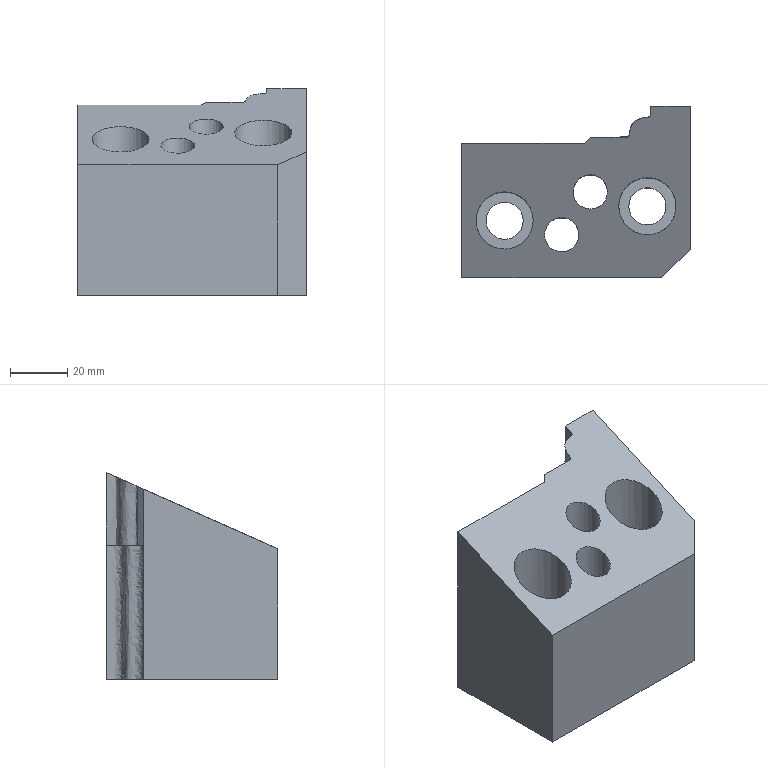Part | NX | features solid 2 | 1 solid | 20 faces | box 80 x 60 x 72.376 mm | volume 180739 mm3 | plane 11 | cylinder 6 | spline 3 | commonest cylinder face diameters 12 x2 13 x2 20 x2
STEP:
#1=CARTESIAN_POINT('',(-526.5,770.,-210.));
#2=VERTEX_POINT('',#1);
#3=CARTESIAN_POINT('',(-533.,770.,-210.));
#4=DIRECTION('',(0.,0.,1.));
#5=DIRECTION('',(1.,0.,0.));
#6=AXIS2_PLACEMENT_3D('',#3,#4,#5);
#7=CIRCLE('',#6,6.5);
#8=EDGE_CURVE('',#2,#2,#7,.F.);
#9=ORIENTED_EDGE('',*,*,#8,.F.);
#10=EDGE_LOOP('',(#9));
#11=FACE_BOUND('',#10,.T.);
#12=CARTESIAN_POINT('',(-476.5,775.,-210.));
#13=VERTEX_POINT('',#12);
#14=CARTESIAN_POINT('',(-483.,775.,-210.));
#15=DIRECTION('',(0.,0.,1.));
#16=DIRECTION('',(1.,0.,0.));
#17=AXIS2_PLACEMENT_3D('',#14,#15,#16);
#18=CIRCLE('',#17,6.5);
#19=EDGE_CURVE('',#13,#13,#18,.F.);
#20=ORIENTED_EDGE('',*,*,#19,.F.);
#21=EDGE_LOOP('',(#20));
#22=FACE_BOUND('',#21,.T.);
#23=CARTESIAN_POINT('',(-497.,780.,-210.));
#24=VERTEX_POINT('',#23);
#25=CARTESIAN_POINT('',(-503.,780.,-210.));
#26=DIRECTION('',(0.,0.,1.));
#27=DIRECTION('',(1.,0.,0.));
#28=AXIS2_PLACEMENT_3D('',#25,#26,#27);
#29=CIRCLE('',#28,6.);
#30=EDGE_CURVE('',#24,#24,#29,.T.);
#31=ORIENTED_EDGE('',*,*,#30,.T.);
#32=EDGE_LOOP('',(#31));
#33=FACE_BOUND('',#32,.T.);
#34=CARTESIAN_POINT('',(-507.,765.,-210.));
#35=VERTEX_POINT('',#34);
#36=CARTESIAN_POINT('',(-513.,765.,-210.));
#37=DIRECTION('',(0.,0.,1.));
#38=DIRECTION('',(1.,0.,0.));
#39=AXIS2_PLACEMENT_3D('',#36,#37,#38);
#40=CIRCLE('',#39,6.);
#41=EDGE_CURVE('',#35,#35,#40,.T.);
#42=ORIENTED_EDGE('',*,*,#41,.T.);
#43=EDGE_LOOP('',(#42));
#44=FACE_BOUND('',#43,.T.);
#45=CARTESIAN_POINT('',(-479.634,810.,-210.));
#46=VERTEX_POINT('',#45);
#47=CARTESIAN_POINT('',(-505.156,797.,-210.));
#48=VERTEX_POINT('',#47);
#49=CARTESIAN_POINT('',(-505.156,797.,-210.));
#50=CARTESIAN_POINT('',(-501.176,797.,-210.));
#51=CARTESIAN_POINT('',(-497.196,797.,-210.));
#52=CARTESIAN_POINT('',(-493.216,797.,-210.));
#53=CARTESIAN_POINT('',(-492.832,797.,-210.));
#54=CARTESIAN_POINT('',(-492.076,797.002,-210.));
#55=CARTESIAN_POINT('',(-491.171,796.978,-210.));
#56=CARTESIAN_POINT('',(-490.387,796.991,-210.));
#57=CARTESIAN_POINT('',(-490.095,797.005,-210.));
#58=CARTESIAN_POINT('',(-489.739,797.026,-210.));
#59=CARTESIAN_POINT('',(-489.186,797.163,-210.));
#60=CARTESIAN_POINT('',(-488.37,797.523,-210.));
#61=CARTESIAN_POINT('',(-487.599,798.274,-210.));
#62=CARTESIAN_POINT('',(-487.195,799.181,-210.));
#63=CARTESIAN_POINT('',(-487.08,799.817,-210.));
#64=CARTESIAN_POINT('',(-487.037,800.426,-210.));
#65=CARTESIAN_POINT('',(-486.999,801.092,-210.));
#66=CARTESIAN_POINT('',(-486.838,801.902,-210.));
#67=CARTESIAN_POINT('',(-486.363,802.737,-210.));
#68=CARTESIAN_POINT('',(-485.47,803.365,-210.));
#69=CARTESIAN_POINT('',(-484.448,803.704,-210.));
#70=CARTESIAN_POINT('',(-483.835,803.806,-210.));
#71=CARTESIAN_POINT('',(-483.198,803.851,-210.));
#72=CARTESIAN_POINT('',(-482.731,803.897,-210.));
#73=CARTESIAN_POINT('',(-482.41,803.93,-210.));
#74=CARTESIAN_POINT('',(-481.63,804.089,-210.));
#75=CARTESIAN_POINT('',(-480.777,804.582,-210.));
#76=CARTESIAN_POINT('',(-480.157,805.239,-210.));
#77=CARTESIAN_POINT('',(-479.718,806.198,-210.));
#78=CARTESIAN_POINT('',(-479.64,806.858,-210.));
#79=CARTESIAN_POINT('',(-479.609,807.399,-210.));
#80=CARTESIAN_POINT('',(-479.625,808.001,-210.));
#81=CARTESIAN_POINT('',(-479.634,808.486,-210.));
#82=CARTESIAN_POINT('',(-479.634,808.867,-210.));
#83=CARTESIAN_POINT('',(-479.634,809.059,-210.));
#84=CARTESIAN_POINT('',(-479.634,809.373,-210.));
#85=CARTESIAN_POINT('',(-479.634,809.686,-210.));
#86=CARTESIAN_POINT('',(-479.634,810.,-210.));
#87=B_SPLINE_CURVE_WITH_KNOTS('',3,(#49,#50,#51,#52,#53,#54,#55,#56,#57,#58,#59,#60,#61,#62,#63,#64,#65,#66,#67,#68,#69,#70,#71,#72,#73,#74,#75,#76,#77,#78,#79,#80,#81,#82,#83,#84,#85,#86),.UNSPECIFIED.,.F.,.F.,(4,3,1,1,1,1,1,1,1,1,1,1,1,1,1,1,1,1,1,1,1,1,1,1,1,1,1,1,1,1,3,4),(0.,0.3484,0.3874,0.4264,0.4459,0.4508,0.4557,0.4605,0.4654,0.4849,0.4947,0.4996,0.5044,0.5434,0.5824,0.6605,0.7385,0.7775,0.8165,0.836,0.8458,0.8555,0.8653,0.875,0.8848,0.8945,0.9043,0.914,0.9335,0.953,0.9725,1.),.UNSPECIFIED.);
#88=EDGE_CURVE('',#46,#48,#87,.F.);
#89=ORIENTED_EDGE('',*,*,#88,.F.);
#90=CARTESIAN_POINT('',(-468.,810.,-210.));
#91=VERTEX_POINT('',#90);
#92=CARTESIAN_POINT('',(-468.,810.,-210.));
#93=DIRECTION('',(-1.,0.,0.));
#94=VECTOR('',#93,1000.);
#95=LINE('',#92,#94);
#96=EDGE_CURVE('',#91,#46,#95,.T.);
#97=ORIENTED_EDGE('',*,*,#96,.F.);
#98=CARTESIAN_POINT('',(-468.,760.,-210.));
#99=VERTEX_POINT('',#98);
#100=CARTESIAN_POINT('',(-468.,750.,-210.));
#101=DIRECTION('',(0.,1.,0.));
#102=VECTOR('',#101,1000.);
#103=LINE('',#100,#102);
#104=EDGE_CURVE('',#99,#91,#103,.T.);
#105=ORIENTED_EDGE('',*,*,#104,.F.);
#106=CARTESIAN_POINT('',(-478.,750.,-210.));
#107=VERTEX_POINT('',#106);
#108=CARTESIAN_POINT('',(-478.,750.,-210.));
#109=DIRECTION('',(-0.7071,-0.7071,0.));
#110=VECTOR('',#109,1000.);
#111=LINE('',#108,#110);
#112=EDGE_CURVE('',#99,#107,#111,.T.);
#113=ORIENTED_EDGE('',*,*,#112,.T.);
#114=CARTESIAN_POINT('',(-548.,750.,-210.));
#115=VERTEX_POINT('',#114);
#116=CARTESIAN_POINT('',(-468.,750.,-210.));
#117=DIRECTION('',(-1.,0.,0.));
#118=VECTOR('',#117,1000.);
#119=LINE('',#116,#118);
#120=EDGE_CURVE('',#107,#115,#119,.T.);
#121=ORIENTED_EDGE('',*,*,#120,.T.);
#122=CARTESIAN_POINT('',(-548.,797.,-210.));
#123=VERTEX_POINT('',#122);
#124=CARTESIAN_POINT('',(-548.,750.,-210.));
#125=DIRECTION('',(0.,1.,0.));
#126=VECTOR('',#125,1000.);
#127=LINE('',#124,#126);
#128=EDGE_CURVE('',#115,#123,#127,.T.);
#129=ORIENTED_EDGE('',*,*,#128,.T.);
#130=CARTESIAN_POINT('',(-505.156,797.,-210.));
#131=DIRECTION('',(-1.,0.,0.));
#132=VECTOR('',#131,1000.);
#133=LINE('',#130,#132);
#134=EDGE_CURVE('',#48,#123,#133,.T.);
#135=ORIENTED_EDGE('',*,*,#134,.F.);
#136=EDGE_LOOP('',(#89,#97,#105,#113,#121,#129,#135));
#137=FACE_BOUND('',#136,.T.);
#138=CARTESIAN_POINT('',(-489.201,800.364,-210.));
#139=DIRECTION('',(0.,0.,1.));
#140=DIRECTION('',(1.,0.,0.));
#141=AXIS2_PLACEMENT_3D('',#138,#139,#140);
#142=PLANE('',#141);
#143=ADVANCED_FACE('',(#11,#22,#33,#44,#137),#142,.F.);
#144=ORIENTED_EDGE('',*,*,#96,.T.);
#145=CARTESIAN_POINT('',(-479.634,810.,-163.));
#146=VERTEX_POINT('',#145);
#147=CARTESIAN_POINT('',(-479.634,810.,-200.));
#148=DIRECTION('',(0.,0.,-1.));
#149=VECTOR('',#148,1000.);
#150=LINE('',#147,#149);
#151=EDGE_CURVE('',#146,#46,#150,.T.);
#152=ORIENTED_EDGE('',*,*,#151,.F.);
#153=CARTESIAN_POINT('',(-481.79,810.,-163.));
#154=VERTEX_POINT('',#153);
#155=CARTESIAN_POINT('',(-481.79,810.,-163.));
#156=DIRECTION('',(1.,0.,0.));
#157=VECTOR('',#156,1000.);
#158=LINE('',#155,#157);
#159=EDGE_CURVE('',#154,#146,#158,.T.);
#160=ORIENTED_EDGE('',*,*,#159,.F.);
#161=CARTESIAN_POINT('',(-481.79,810.,-137.624));
#162=VERTEX_POINT('',#161);
#163=CARTESIAN_POINT('',(-481.79,810.,-210.));
#164=DIRECTION('',(0.,0.,1.));
#165=VECTOR('',#164,1000.);
#166=LINE('',#163,#165);
#167=EDGE_CURVE('',#154,#162,#166,.T.);
#168=ORIENTED_EDGE('',*,*,#167,.T.);
#169=CARTESIAN_POINT('',(-468.,810.,-137.624));
#170=VERTEX_POINT('',#169);
#171=CARTESIAN_POINT('',(-468.,810.,-137.624));
#172=DIRECTION('',(1.,0.,0.));
#173=VECTOR('',#172,1000.);
#174=LINE('',#171,#173);
#175=EDGE_CURVE('',#162,#170,#174,.T.);
#176=ORIENTED_EDGE('',*,*,#175,.T.);
#177=CARTESIAN_POINT('',(-468.,810.,-210.));
#178=DIRECTION('',(0.,0.,1.));
#179=VECTOR('',#178,1000.);
#180=LINE('',#177,#179);
#181=EDGE_CURVE('',#91,#170,#180,.T.);
#182=ORIENTED_EDGE('',*,*,#181,.F.);
#183=EDGE_LOOP('',(#144,#152,#160,#168,#176,#182));
#184=FACE_BOUND('',#183,.T.);
#185=CARTESIAN_POINT('',(-468.,810.,-210.));
#186=DIRECTION('',(0.,1.,0.));
#187=DIRECTION('',(0.,0.,1.));
#188=AXIS2_PLACEMENT_3D('',#185,#186,#187);
#189=PLANE('',#188);
#190=ADVANCED_FACE('',(#184),#189,.T.);
#191=CARTESIAN_POINT('',(-503.,799.156,-163.));
#192=VERTEX_POINT('',#191);
#193=CARTESIAN_POINT('',(-503.,799.156,-163.));
#194=CARTESIAN_POINT('',(-501.803,799.156,-163.));
#195=CARTESIAN_POINT('',(-499.409,799.156,-163.));
#196=CARTESIAN_POINT('',(-496.416,799.156,-163.));
#197=CARTESIAN_POINT('',(-494.021,799.155,-163.));
#198=CARTESIAN_POINT('',(-492.527,799.158,-163.));
#199=CARTESIAN_POINT('',(-491.326,799.147,-163.));
#200=CARTESIAN_POINT('',(-490.443,799.121,-163.));
#201=CARTESIAN_POINT('',(-489.489,799.261,-163.));
#202=CARTESIAN_POINT('',(-489.159,800.175,-163.));
#203=CARTESIAN_POINT('',(-489.173,801.069,-163.));
#204=CARTESIAN_POINT('',(-488.995,802.265,-163.));
#205=CARTESIAN_POINT('',(-488.407,803.667,-163.));
#206=CARTESIAN_POINT('',(-487.101,804.952,-163.));
#207=CARTESIAN_POINT('',(-485.449,805.72,-163.));
#208=CARTESIAN_POINT('',(-483.973,805.988,-163.));
#209=CARTESIAN_POINT('',(-482.783,806.009,-163.));
#210=CARTESIAN_POINT('',(-481.868,806.352,-163.));
#211=CARTESIAN_POINT('',(-481.749,807.326,-163.));
#212=CARTESIAN_POINT('',(-481.806,808.496,-163.));
#213=CARTESIAN_POINT('',(-481.79,809.402,-163.));
#214=CARTESIAN_POINT('',(-481.79,810.,-163.));
#215=B_SPLINE_CURVE_WITH_KNOTS('',3,(#193,#194,#195,#196,#197,#198,#199,#200,#201,#202,#203,#204,#205,#206,#207,#208,#209,#210,#211,#212,#213,#214),.UNSPECIFIED.,.F.,.F.,(4,1,1,1,1,1,1,1,1,1,1,1,1,1,1,1,1,1,1,4),(0.1166,0.1202,0.1238,0.1256,0.1274,0.1283,0.1292,0.1301,0.131,0.1319,0.1328,0.1346,0.1364,0.1382,0.14,0.1409,0.1418,0.1427,0.1436,0.1453),.UNSPECIFIED.);
#216=EDGE_CURVE('',#154,#192,#215,.F.);
#217=ORIENTED_EDGE('',*,*,#216,.T.);
#218=CARTESIAN_POINT('',(-503.,799.156,-142.439));
#219=VERTEX_POINT('',#218);
#220=CARTESIAN_POINT('',(-503.,799.156,-210.));
#221=DIRECTION('',(0.,0.,1.));
#222=VECTOR('',#221,1000.);
#223=LINE('',#220,#222);
#224=EDGE_CURVE('',#192,#219,#223,.T.);
#225=ORIENTED_EDGE('',*,*,#224,.T.);
#226=CARTESIAN_POINT('',(-481.79,810.,-137.624));
#227=CARTESIAN_POINT('',(-481.79,809.471,-137.859));
#228=CARTESIAN_POINT('',(-481.792,808.677,-138.212));
#229=CARTESIAN_POINT('',(-481.779,807.619,-138.681));
#230=CARTESIAN_POINT('',(-481.73,806.822,-139.035));
#231=CARTESIAN_POINT('',(-482.268,806.06,-139.374));
#232=CARTESIAN_POINT('',(-483.235,806.021,-139.391));
#233=CARTESIAN_POINT('',(-484.125,805.946,-139.424));
#234=CARTESIAN_POINT('',(-485.303,805.732,-139.519));
#235=CARTESIAN_POINT('',(-486.698,805.191,-139.759));
#236=CARTESIAN_POINT('',(-488.068,804.085,-140.25));
#237=CARTESIAN_POINT('',(-488.93,802.607,-140.906));
#238=CARTESIAN_POINT('',(-489.165,801.24,-141.513));
#239=CARTESIAN_POINT('',(-489.185,800.27,-141.944));
#240=CARTESIAN_POINT('',(-489.293,799.723,-142.187));
#241=CARTESIAN_POINT('',(-489.585,799.349,-142.353));
#242=CARTESIAN_POINT('',(-490.021,799.141,-142.445));
#243=CARTESIAN_POINT('',(-490.672,799.149,-142.442));
#244=CARTESIAN_POINT('',(-491.468,799.142,-142.445));
#245=CARTESIAN_POINT('',(-492.43,799.158,-142.438));
#246=CARTESIAN_POINT('',(-493.711,799.155,-142.439));
#247=CARTESIAN_POINT('',(-495.313,799.156,-142.438));
#248=CARTESIAN_POINT('',(-497.234,799.156,-142.439));
#249=CARTESIAN_POINT('',(-499.797,799.156,-142.439));
#250=CARTESIAN_POINT('',(-501.719,799.156,-142.439));
#251=CARTESIAN_POINT('',(-503.,799.156,-142.439));
#252=B_SPLINE_CURVE_WITH_KNOTS('',3,(#226,#227,#228,#229,#230,#231,#232,#233,#234,#235,#236,#237,#238,#239,#240,#241,#242,#243,#244,#245,#246,#247,#248,#249,#250,#251),.UNSPECIFIED.,.F.,.F.,(4,1,1,1,1,1,1,1,1,1,1,1,1,1,1,1,1,1,1,1,1,1,1,4),(0.,0.001737,0.002605,0.003474,0.004342,0.005211,0.006079,0.006948,0.008684,0.01042,0.01216,0.0139,0.01476,0.0152,0.01563,0.01607,0.0165,0.01737,0.01824,0.01911,0.02084,0.02258,0.02432,0.02779),.UNSPECIFIED.);
#253=EDGE_CURVE('',#162,#219,#252,.T.);
#254=ORIENTED_EDGE('',*,*,#253,.F.);
#255=ORIENTED_EDGE('',*,*,#167,.F.);
#256=EDGE_LOOP('',(#217,#225,#254,#255));
#257=FACE_BOUND('',#256,.T.);
#258=CARTESIAN_POINT('',(-503.,799.156,-163.));
#259=CARTESIAN_POINT('',(-503.,799.156,-137.472));
#260=CARTESIAN_POINT('',(-501.785,799.156,-163.));
#261=CARTESIAN_POINT('',(-501.785,799.156,-137.472));
#262=CARTESIAN_POINT('',(-499.356,799.156,-163.));
#263=CARTESIAN_POINT('',(-499.356,799.156,-137.472));
#264=CARTESIAN_POINT('',(-496.319,799.156,-163.));
#265=CARTESIAN_POINT('',(-496.319,799.156,-137.472));
#266=CARTESIAN_POINT('',(-494.193,799.156,-163.));
#267=CARTESIAN_POINT('',(-494.193,799.156,-137.472));
#268=CARTESIAN_POINT('',(-492.978,799.156,-163.));
#269=CARTESIAN_POINT('',(-492.978,799.156,-137.472));
#270=CARTESIAN_POINT('',(-492.066,799.155,-163.));
#271=CARTESIAN_POINT('',(-492.066,799.155,-137.472));
#272=CARTESIAN_POINT('',(-491.154,799.143,-163.));
#273=CARTESIAN_POINT('',(-491.154,799.143,-137.472));
#274=CARTESIAN_POINT('',(-490.394,799.127,-163.));
#275=CARTESIAN_POINT('',(-490.394,799.127,-137.472));
#276=CARTESIAN_POINT('',(-489.79,799.213,-163.));
#277=CARTESIAN_POINT('',(-489.79,799.213,-137.472));
#278=CARTESIAN_POINT('',(-489.428,799.513,-163.));
#279=CARTESIAN_POINT('',(-489.428,799.513,-137.472));
#280=CARTESIAN_POINT('',(-489.219,799.933,-163.));
#281=CARTESIAN_POINT('',(-489.219,799.933,-137.472));
#282=CARTESIAN_POINT('',(-489.197,800.51,-163.));
#283=CARTESIAN_POINT('',(-489.197,800.51,-137.472));
#284=CARTESIAN_POINT('',(-489.145,801.213,-163.));
#285=CARTESIAN_POINT('',(-489.145,801.213,-137.472));
#286=CARTESIAN_POINT('',(-488.978,802.326,-163.));
#287=CARTESIAN_POINT('',(-488.978,802.326,-137.472));
#288=CARTESIAN_POINT('',(-488.407,803.64,-163.));
#289=CARTESIAN_POINT('',(-488.407,803.64,-137.472));
#290=CARTESIAN_POINT('',(-487.178,804.894,-163.));
#291=CARTESIAN_POINT('',(-487.178,804.894,-137.472));
#292=CARTESIAN_POINT('',(-485.556,805.688,-163.));
#293=CARTESIAN_POINT('',(-485.556,805.688,-137.472));
#294=CARTESIAN_POINT('',(-484.055,805.979,-163.));
#295=CARTESIAN_POINT('',(-484.055,805.979,-137.472));
#296=CARTESIAN_POINT('',(-482.852,806.011,-163.));
#297=CARTESIAN_POINT('',(-482.852,806.011,-137.472));
#298=CARTESIAN_POINT('',(-481.905,806.299,-163.));
#299=CARTESIAN_POINT('',(-481.905,806.299,-137.472));
#300=CARTESIAN_POINT('',(-481.742,807.279,-163.));
#301=CARTESIAN_POINT('',(-481.742,807.279,-137.472));
#302=CARTESIAN_POINT('',(-481.809,808.473,-163.));
#303=CARTESIAN_POINT('',(-481.809,808.473,-137.472));
#304=CARTESIAN_POINT('',(-481.79,809.393,-163.));
#305=CARTESIAN_POINT('',(-481.79,809.393,-137.472));
#306=CARTESIAN_POINT('',(-481.79,810.,-163.));
#307=CARTESIAN_POINT('',(-481.79,810.,-137.472));
#308=B_SPLINE_SURFACE_WITH_KNOTS('',3,1,((#258,#259),(#260,#261),(#262,#263),(#264,#265),(#266,#267),(#268,#269),(#270,#271),(#272,#273),(#274,#275),(#276,#277),(#278,#279),(#280,#281),(#282,#283),(#284,#285),(#286,#287),(#288,#289),(#290,#291),(#292,#293),(#294,#295),(#296,#297),(#298,#299),(#300,#301),(#302,#303),(#304,#305),(#306,#307)),.SURF_OF_LINEAR_EXTRUSION.,.F.,.F.,.F.,(4,1,1,1,1,1,1,1,1,1,1,1,1,1,1,1,1,1,1,1,1,1,4),(2,2),(0.,0.125,0.25,0.3125,0.3437,0.375,0.4062,0.4375,0.4531,0.4687,0.4844,0.5,0.5312,0.5625,0.625,0.6875,0.75,0.8125,0.8437,0.875,0.9062,0.9375,1.),(0.,1.),.UNSPECIFIED.);
#309=ADVANCED_FACE('',(#257),#308,.F.);
#310=CARTESIAN_POINT('',(-507.,765.,-157.603));
#311=VERTEX_POINT('',#310);
#312=CARTESIAN_POINT('',(-507.877,761.22,-159.281));
#313=CARTESIAN_POINT('',(-506.424,765.002,-157.602));
#314=CARTESIAN_POINT('',(-508.136,769.527,-155.593));
#315=CARTESIAN_POINT('',(-512.977,771.731,-154.614));
#316=CARTESIAN_POINT('',(-517.857,769.547,-155.584));
#317=CARTESIAN_POINT('',(-519.57,765.007,-157.6));
#318=CARTESIAN_POINT('',(-517.864,760.475,-159.612));
#319=CARTESIAN_POINT('',(-513.86,758.647,-160.424));
#320=CARTESIAN_POINT('',(-510.549,759.34,-160.116));
#321=CARTESIAN_POINT('',(-507.877,761.22,-159.281));
#322=CARTESIAN_POINT('',(-506.424,765.002,-157.602));
#323=CARTESIAN_POINT('',(-508.136,769.527,-155.593));
#324=B_SPLINE_CURVE_WITH_KNOTS('',3,(#312,#313,#314,#315,#316,#317,#318,#319,#320,#321,#322,#323),.UNSPECIFIED.,.T.,.F.,(1,1,1,1,1,1,1,1,1,1,1,1,1,1,1,1),(-0.00981,-0.007358,-0.004905,0.,0.004905,0.00981,0.01472,0.01962,0.02453,0.02943,0.03188,0.03434,0.03924,0.04415,0.04905,0.05396),.UNSPECIFIED.);
#325=EDGE_CURVE('',#311,#311,#324,.T.);
#326=ORIENTED_EDGE('',*,*,#325,.F.);
#327=EDGE_LOOP('',(#326));
#328=FACE_BOUND('',#327,.T.);
#329=CARTESIAN_POINT('',(-497.,780.,-150.943));
#330=VERTEX_POINT('',#329);
#331=CARTESIAN_POINT('',(-497.877,776.22,-152.622));
#332=CARTESIAN_POINT('',(-496.424,780.002,-150.942));
#333=CARTESIAN_POINT('',(-498.136,784.527,-148.933));
#334=CARTESIAN_POINT('',(-502.977,786.731,-147.955));
#335=CARTESIAN_POINT('',(-507.857,784.547,-148.925));
#336=CARTESIAN_POINT('',(-509.57,780.007,-150.94));
#337=CARTESIAN_POINT('',(-507.864,775.475,-152.952));
#338=CARTESIAN_POINT('',(-503.86,773.647,-153.764));
#339=CARTESIAN_POINT('',(-500.549,774.34,-153.456));
#340=CARTESIAN_POINT('',(-497.877,776.22,-152.622));
#341=CARTESIAN_POINT('',(-496.424,780.002,-150.942));
#342=CARTESIAN_POINT('',(-498.136,784.527,-148.933));
#343=B_SPLINE_CURVE_WITH_KNOTS('',3,(#331,#332,#333,#334,#335,#336,#337,#338,#339,#340,#341,#342),.UNSPECIFIED.,.T.,.F.,(1,1,1,1,1,1,1,1,1,1,1,1,1,1,1,1),(-0.00981,-0.007358,-0.004905,0.,0.004905,0.00981,0.01472,0.01962,0.02453,0.02943,0.03188,0.03434,0.03924,0.04415,0.04905,0.05396),.UNSPECIFIED.);
#344=EDGE_CURVE('',#330,#330,#343,.T.);
#345=ORIENTED_EDGE('',*,*,#344,.F.);
#346=EDGE_LOOP('',(#345));
#347=FACE_BOUND('',#346,.T.);
#348=CARTESIAN_POINT('',(-523.,770.,-155.383));
#349=VERTEX_POINT('',#348);
#350=CARTESIAN_POINT('',(-524.462,763.701,-158.18));
#351=CARTESIAN_POINT('',(-522.029,770.009,-155.379));
#352=CARTESIAN_POINT('',(-524.451,776.271,-152.599));
#353=CARTESIAN_POINT('',(-528.869,779.412,-151.204));
#354=CARTESIAN_POINT('',(-532.971,780.288,-150.815));
#355=CARTESIAN_POINT('',(-537.082,779.435,-151.194));
#356=CARTESIAN_POINT('',(-541.538,776.297,-152.587));
#357=CARTESIAN_POINT('',(-543.968,770.011,-155.378));
#358=CARTESIAN_POINT('',(-541.557,763.738,-158.163));
#359=CARTESIAN_POINT('',(-537.142,760.594,-159.559));
#360=CARTESIAN_POINT('',(-533.043,759.711,-159.951));
#361=CARTESIAN_POINT('',(-528.917,760.564,-159.572));
#362=CARTESIAN_POINT('',(-524.462,763.701,-158.18));
#363=CARTESIAN_POINT('',(-522.029,770.009,-155.379));
#364=CARTESIAN_POINT('',(-524.451,776.271,-152.599));
#365=B_SPLINE_CURVE_WITH_KNOTS('',3,(#350,#351,#352,#353,#354,#355,#356,#357,#358,#359,#360,#361,#362,#363,#364),.UNSPECIFIED.,.T.,.F.,(1,1,1,1,1,1,1,1,1,1,1,1,1,1,1,1,1,1,1),(-0.01635,-0.01226,-0.008175,0.,0.008175,0.01226,0.01635,0.02044,0.02453,0.0327,0.04088,0.04496,0.04905,0.05314,0.05723,0.0654,0.07358,0.07766,0.08175),.UNSPECIFIED.);
#366=EDGE_CURVE('',#349,#349,#365,.T.);
#367=ORIENTED_EDGE('',*,*,#366,.F.);
#368=EDGE_LOOP('',(#367));
#369=FACE_BOUND('',#368,.T.);
#370=CARTESIAN_POINT('',(-473.,775.,-153.163));
#371=VERTEX_POINT('',#370);
#372=CARTESIAN_POINT('',(-474.462,768.701,-155.96));
#373=CARTESIAN_POINT('',(-472.029,775.009,-153.159));
#374=CARTESIAN_POINT('',(-474.451,781.271,-150.379));
#375=CARTESIAN_POINT('',(-478.869,784.412,-148.985));
#376=CARTESIAN_POINT('',(-482.971,785.288,-148.596));
#377=CARTESIAN_POINT('',(-487.082,784.435,-148.974));
#378=CARTESIAN_POINT('',(-491.538,781.297,-150.367));
#379=CARTESIAN_POINT('',(-493.968,775.011,-153.158));
#380=CARTESIAN_POINT('',(-491.557,768.738,-155.943));
#381=CARTESIAN_POINT('',(-487.142,765.594,-157.339));
#382=CARTESIAN_POINT('',(-483.043,764.711,-157.732));
#383=CARTESIAN_POINT('',(-478.917,765.564,-157.353));
#384=CARTESIAN_POINT('',(-474.462,768.701,-155.96));
#385=CARTESIAN_POINT('',(-472.029,775.009,-153.159));
#386=CARTESIAN_POINT('',(-474.451,781.271,-150.379));
#387=B_SPLINE_CURVE_WITH_KNOTS('',3,(#372,#373,#374,#375,#376,#377,#378,#379,#380,#381,#382,#383,#384,#385,#386),.UNSPECIFIED.,.T.,.F.,(1,1,1,1,1,1,1,1,1,1,1,1,1,1,1,1,1,1,1),(-0.01635,-0.01226,-0.008175,0.,0.008175,0.01226,0.01635,0.02044,0.02453,0.0327,0.04088,0.04496,0.04905,0.05314,0.05723,0.0654,0.07358,0.07766,0.08175),.UNSPECIFIED.);
#388=EDGE_CURVE('',#371,#371,#387,.T.);
#389=ORIENTED_EDGE('',*,*,#388,.F.);
#390=EDGE_LOOP('',(#389));
#391=FACE_BOUND('',#390,.T.);
#392=CARTESIAN_POINT('',(-548.,750.,-164.263));
#393=VERTEX_POINT('',#392);
#394=CARTESIAN_POINT('',(-478.,750.,-164.263));
#395=VERTEX_POINT('',#394);
#396=CARTESIAN_POINT('',(-468.,750.,-164.263));
#397=DIRECTION('',(1.,0.,0.));
#398=VECTOR('',#397,1000.);
#399=LINE('',#396,#398);
#400=EDGE_CURVE('',#393,#395,#399,.T.);
#401=ORIENTED_EDGE('',*,*,#400,.T.);
#402=CARTESIAN_POINT('',(-468.,760.,-159.823));
#403=VERTEX_POINT('',#402);
#404=CARTESIAN_POINT('',(-478.,750.,-164.263));
#405=CARTESIAN_POINT('',(-474.667,753.333,-162.783));
#406=CARTESIAN_POINT('',(-471.333,756.667,-161.303));
#407=CARTESIAN_POINT('',(-468.,760.,-159.823));
#408=B_SPLINE_CURVE_WITH_KNOTS('',3,(#404,#405,#406,#407),.UNSPECIFIED.,.F.,.F.,(4,4),(0.,0.01482),.UNSPECIFIED.);
#409=EDGE_CURVE('',#395,#403,#408,.T.);
#410=ORIENTED_EDGE('',*,*,#409,.T.);
#411=CARTESIAN_POINT('',(-468.,733.037,-171.794));
#412=DIRECTION('',(0.,-0.914,-0.4058));
#413=VECTOR('',#412,1000.);
#414=LINE('',#411,#413);
#415=EDGE_CURVE('',#170,#403,#414,.T.);
#416=ORIENTED_EDGE('',*,*,#415,.F.);
#417=ORIENTED_EDGE('',*,*,#175,.F.);
#418=ORIENTED_EDGE('',*,*,#253,.T.);
#419=CARTESIAN_POINT('',(-505.156,797.,-143.396));
#420=VERTEX_POINT('',#419);
#421=CARTESIAN_POINT('',(-516.652,785.504,-148.5));
#422=DIRECTION('',(0.6746,0.6746,0.2995));
#423=VECTOR('',#422,1000.);
#424=LINE('',#421,#423);
#425=EDGE_CURVE('',#420,#219,#424,.T.);
#426=ORIENTED_EDGE('',*,*,#425,.F.);
#427=CARTESIAN_POINT('',(-548.,797.,-143.396));
#428=VERTEX_POINT('',#427);
#429=CARTESIAN_POINT('',(-505.156,797.,-143.396));
#430=DIRECTION('',(1.,0.,0.));
#431=VECTOR('',#430,1000.);
#432=LINE('',#429,#431);
#433=EDGE_CURVE('',#428,#420,#432,.T.);
#434=ORIENTED_EDGE('',*,*,#433,.F.);
#435=CARTESIAN_POINT('',(-548.,733.037,-171.794));
#436=DIRECTION('',(0.,-0.914,-0.4058));
#437=VECTOR('',#436,1000.);
#438=LINE('',#435,#437);
#439=EDGE_CURVE('',#428,#393,#438,.T.);
#440=ORIENTED_EDGE('',*,*,#439,.T.);
#441=EDGE_LOOP('',(#401,#410,#416,#417,#418,#426,#434,#440));
#442=FACE_BOUND('',#441,.T.);
#443=CARTESIAN_POINT('',(-548.,810.,-137.624));
#444=CARTESIAN_POINT('',(-468.,810.,-137.624));
#445=CARTESIAN_POINT('',(-548.,750.,-164.263));
#446=CARTESIAN_POINT('',(-468.,750.,-164.263));
#447=B_SPLINE_SURFACE_WITH_KNOTS('',1,1,((#443,#444),(#445,#446)),.PLANE_SURF.,.F.,.F.,.F.,(2,2),(2,2),(0.3497,0.4444),(0.2449,0.5614),.PIECEWISE_BEZIER_KNOTS.);
#448=ADVANCED_FACE('',(#328,#347,#369,#391,#442),#447,.T.);
#449=CARTESIAN_POINT('',(-548.,797.,-210.));
#450=DIRECTION('',(0.,0.,1.));
#451=VECTOR('',#450,1000.);
#452=LINE('',#449,#451);
#453=EDGE_CURVE('',#123,#428,#452,.T.);
#454=ORIENTED_EDGE('',*,*,#453,.T.);
#455=ORIENTED_EDGE('',*,*,#433,.T.);
#456=CARTESIAN_POINT('',(-505.156,797.,-163.));
#457=VERTEX_POINT('',#456);
#458=CARTESIAN_POINT('',(-505.156,797.,-210.));
#459=DIRECTION('',(0.,0.,1.));
#460=VECTOR('',#459,1000.);
#461=LINE('',#458,#460);
#462=EDGE_CURVE('',#457,#420,#461,.T.);
#463=ORIENTED_EDGE('',*,*,#462,.F.);
#464=CARTESIAN_POINT('',(-505.156,797.,-210.));
#465=DIRECTION('',(0.,0.,1.));
#466=VECTOR('',#465,1000.);
#467=LINE('',#464,#466);
#468=EDGE_CURVE('',#48,#457,#467,.T.);
#469=ORIENTED_EDGE('',*,*,#468,.F.);
#470=ORIENTED_EDGE('',*,*,#134,.T.);
#471=EDGE_LOOP('',(#454,#455,#463,#469,#470));
#472=FACE_BOUND('',#471,.T.);
#473=CARTESIAN_POINT('',(-505.156,797.,-210.));
#474=DIRECTION('',(0.,1.,0.));
#475=DIRECTION('',(0.,0.,1.));
#476=AXIS2_PLACEMENT_3D('',#473,#474,#475);
#477=PLANE('',#476);
#478=ADVANCED_FACE('',(#472),#477,.T.);
#479=ORIENTED_EDGE('',*,*,#439,.F.);
#480=ORIENTED_EDGE('',*,*,#453,.F.);
#481=ORIENTED_EDGE('',*,*,#128,.F.);
#482=CARTESIAN_POINT('',(-548.,750.,-210.));
#483=DIRECTION('',(0.,0.,1.));
#484=VECTOR('',#483,1000.);
#485=LINE('',#482,#484);
#486=EDGE_CURVE('',#115,#393,#485,.T.);
#487=ORIENTED_EDGE('',*,*,#486,.T.);
#488=EDGE_LOOP('',(#479,#480,#481,#487));
#489=FACE_BOUND('',#488,.T.);
#490=CARTESIAN_POINT('',(-548.,750.,-210.));
#491=DIRECTION('',(1.,0.,0.));
#492=DIRECTION('',(0.,0.,-1.));
#493=AXIS2_PLACEMENT_3D('',#490,#491,#492);
#494=PLANE('',#493);
#495=ADVANCED_FACE('',(#489),#494,.F.);
#496=ORIENTED_EDGE('',*,*,#120,.F.);
#497=CARTESIAN_POINT('',(-478.,750.,-164.263));
#498=DIRECTION('',(0.,0.,1.));
#499=VECTOR('',#498,1000.);
#500=LINE('',#497,#499);
#501=EDGE_CURVE('',#107,#395,#500,.T.);
#502=ORIENTED_EDGE('',*,*,#501,.T.);
#503=ORIENTED_EDGE('',*,*,#400,.F.);
#504=ORIENTED_EDGE('',*,*,#486,.F.);
#505=EDGE_LOOP('',(#496,#502,#503,#504));
#506=FACE_BOUND('',#505,.T.);
#507=CARTESIAN_POINT('',(-468.,750.,-210.));
#508=DIRECTION('',(0.,1.,0.));
#509=DIRECTION('',(0.,0.,1.));
#510=AXIS2_PLACEMENT_3D('',#507,#508,#509);
#511=PLANE('',#510);
#512=ADVANCED_FACE('',(#506),#511,.F.);
#513=ORIENTED_EDGE('',*,*,#415,.T.);
#514=CARTESIAN_POINT('',(-468.,760.,-210.));
#515=DIRECTION('',(0.,0.,-1.));
#516=VECTOR('',#515,1000.);
#517=LINE('',#514,#516);
#518=EDGE_CURVE('',#403,#99,#517,.T.);
#519=ORIENTED_EDGE('',*,*,#518,.T.);
#520=ORIENTED_EDGE('',*,*,#104,.T.);
#521=ORIENTED_EDGE('',*,*,#181,.T.);
#522=EDGE_LOOP('',(#513,#519,#520,#521));
#523=FACE_BOUND('',#522,.T.);
#524=CARTESIAN_POINT('',(-468.,750.,-210.));
#525=DIRECTION('',(1.,0.,0.));
#526=DIRECTION('',(0.,0.,-1.));
#527=AXIS2_PLACEMENT_3D('',#524,#525,#526);
#528=PLANE('',#527);
#529=ADVANCED_FACE('',(#523),#528,.T.);
#530=CARTESIAN_POINT('',(-486.973,815.183,-163.));
#531=DIRECTION('',(0.7071,0.7071,0.));
#532=VECTOR('',#531,1000.);
#533=LINE('',#530,#532);
#534=EDGE_CURVE('',#457,#192,#533,.T.);
#535=ORIENTED_EDGE('',*,*,#534,.F.);
#536=ORIENTED_EDGE('',*,*,#462,.T.);
#537=ORIENTED_EDGE('',*,*,#425,.T.);
#538=ORIENTED_EDGE('',*,*,#224,.F.);
#539=EDGE_LOOP('',(#535,#536,#537,#538));
#540=FACE_BOUND('',#539,.T.);
#541=CARTESIAN_POINT('',(-503.,799.156,-210.));
#542=DIRECTION('',(-0.7071,0.7071,0.));
#543=DIRECTION('',(-0.7071,-0.7071,0.));
#544=AXIS2_PLACEMENT_3D('',#541,#542,#543);
#545=PLANE('',#544);
#546=ADVANCED_FACE('',(#540),#545,.T.);
#547=ORIENTED_EDGE('',*,*,#112,.F.);
#548=ORIENTED_EDGE('',*,*,#518,.F.);
#549=ORIENTED_EDGE('',*,*,#409,.F.);
#550=ORIENTED_EDGE('',*,*,#501,.F.);
#551=EDGE_LOOP('',(#547,#548,#549,#550));
#552=FACE_BOUND('',#551,.T.);
#553=CARTESIAN_POINT('',(-478.,750.,-210.));
#554=DIRECTION('',(0.7071,-0.7071,0.));
#555=DIRECTION('',(0.7071,0.7071,0.));
#556=AXIS2_PLACEMENT_3D('',#553,#554,#555);
#557=PLANE('',#556);
#558=ADVANCED_FACE('',(#552),#557,.T.);
#559=CARTESIAN_POINT('',(-476.5,775.,-195.));
#560=VERTEX_POINT('',#559);
#561=CARTESIAN_POINT('',(-483.,775.,-195.));
#562=DIRECTION('',(0.,0.,1.));
#563=DIRECTION('',(1.,0.,0.));
#564=AXIS2_PLACEMENT_3D('',#561,#562,#563);
#565=CIRCLE('',#564,6.5);
#566=EDGE_CURVE('',#560,#560,#565,.T.);
#567=ORIENTED_EDGE('',*,*,#566,.T.);
#568=EDGE_LOOP('',(#567));
#569=FACE_BOUND('',#568,.T.);
#570=ORIENTED_EDGE('',*,*,#19,.T.);
#571=EDGE_LOOP('',(#570));
#572=FACE_BOUND('',#571,.T.);
#573=CARTESIAN_POINT('',(-483.,775.,-195.));
#574=DIRECTION('',(0.,0.,-1.));
#575=DIRECTION('',(-1.,0.,0.));
#576=AXIS2_PLACEMENT_3D('',#573,#574,#575);
#577=CYLINDRICAL_SURFACE('',#576,6.5);
#578=ADVANCED_FACE('',(#569,#572),#577,.F.);
#579=CARTESIAN_POINT('',(-526.5,770.,-195.));
#580=VERTEX_POINT('',#579);
#581=CARTESIAN_POINT('',(-533.,770.,-195.));
#582=DIRECTION('',(0.,0.,1.));
#583=DIRECTION('',(1.,0.,0.));
#584=AXIS2_PLACEMENT_3D('',#581,#582,#583);
#585=CIRCLE('',#584,6.5);
#586=EDGE_CURVE('',#580,#580,#585,.T.);
#587=ORIENTED_EDGE('',*,*,#586,.T.);
#588=EDGE_LOOP('',(#587));
#589=FACE_BOUND('',#588,.T.);
#590=ORIENTED_EDGE('',*,*,#8,.T.);
#591=EDGE_LOOP('',(#590));
#592=FACE_BOUND('',#591,.T.);
#593=CARTESIAN_POINT('',(-533.,770.,-195.));
#594=DIRECTION('',(0.,0.,-1.));
#595=DIRECTION('',(-1.,0.,0.));
#596=AXIS2_PLACEMENT_3D('',#593,#594,#595);
#597=CYLINDRICAL_SURFACE('',#596,6.5);
#598=ADVANCED_FACE('',(#589,#592),#597,.F.);
#599=ORIENTED_EDGE('',*,*,#388,.T.);
#600=EDGE_LOOP('',(#599));
#601=FACE_BOUND('',#600,.T.);
#602=CARTESIAN_POINT('',(-473.,775.,-195.));
#603=VERTEX_POINT('',#602);
#604=CARTESIAN_POINT('',(-483.,775.,-195.));
#605=DIRECTION('',(0.,0.,1.));
#606=DIRECTION('',(1.,0.,0.));
#607=AXIS2_PLACEMENT_3D('',#604,#605,#606);
#608=CIRCLE('',#607,10.);
#609=EDGE_CURVE('',#603,#603,#608,.T.);
#610=ORIENTED_EDGE('',*,*,#609,.F.);
#611=EDGE_LOOP('',(#610));
#612=FACE_BOUND('',#611,.T.);
#613=CARTESIAN_POINT('',(-483.,775.,-195.));
#614=DIRECTION('',(0.,0.,1.));
#615=DIRECTION('',(1.,0.,0.));
#616=AXIS2_PLACEMENT_3D('',#613,#614,#615);
#617=CYLINDRICAL_SURFACE('',#616,10.);
#618=ADVANCED_FACE('',(#601,#612),#617,.F.);
#619=ORIENTED_EDGE('',*,*,#566,.F.);
#620=EDGE_LOOP('',(#619));
#621=FACE_BOUND('',#620,.T.);
#622=ORIENTED_EDGE('',*,*,#609,.T.);
#623=EDGE_LOOP('',(#622));
#624=FACE_BOUND('',#623,.T.);
#625=CARTESIAN_POINT('',(-483.,775.,-195.));
#626=DIRECTION('',(0.,0.,1.));
#627=DIRECTION('',(1.,0.,0.));
#628=AXIS2_PLACEMENT_3D('',#625,#626,#627);
#629=PLANE('',#628);
#630=ADVANCED_FACE('',(#621,#624),#629,.T.);
#631=ORIENTED_EDGE('',*,*,#366,.T.);
#632=EDGE_LOOP('',(#631));
#633=FACE_BOUND('',#632,.T.);
#634=CARTESIAN_POINT('',(-523.,770.,-195.));
#635=VERTEX_POINT('',#634);
#636=CARTESIAN_POINT('',(-533.,770.,-195.));
#637=DIRECTION('',(0.,0.,1.));
#638=DIRECTION('',(1.,0.,0.));
#639=AXIS2_PLACEMENT_3D('',#636,#637,#638);
#640=CIRCLE('',#639,10.);
#641=EDGE_CURVE('',#635,#635,#640,.T.);
#642=ORIENTED_EDGE('',*,*,#641,.F.);
#643=EDGE_LOOP('',(#642));
#644=FACE_BOUND('',#643,.T.);
#645=CARTESIAN_POINT('',(-533.,770.,-195.));
#646=DIRECTION('',(0.,0.,1.));
#647=DIRECTION('',(1.,0.,0.));
#648=AXIS2_PLACEMENT_3D('',#645,#646,#647);
#649=CYLINDRICAL_SURFACE('',#648,10.);
#650=ADVANCED_FACE('',(#633,#644),#649,.F.);
#651=ORIENTED_EDGE('',*,*,#586,.F.);
#652=EDGE_LOOP('',(#651));
#653=FACE_BOUND('',#652,.T.);
#654=ORIENTED_EDGE('',*,*,#641,.T.);
#655=EDGE_LOOP('',(#654));
#656=FACE_BOUND('',#655,.T.);
#657=CARTESIAN_POINT('',(-533.,770.,-195.));
#658=DIRECTION('',(0.,0.,1.));
#659=DIRECTION('',(1.,0.,0.));
#660=AXIS2_PLACEMENT_3D('',#657,#658,#659);
#661=PLANE('',#660);
#662=ADVANCED_FACE('',(#653,#656),#661,.T.);
#663=ORIENTED_EDGE('',*,*,#344,.T.);
#664=EDGE_LOOP('',(#663));
#665=FACE_BOUND('',#664,.T.);
#666=ORIENTED_EDGE('',*,*,#30,.F.);
#667=EDGE_LOOP('',(#666));
#668=FACE_BOUND('',#667,.T.);
#669=CARTESIAN_POINT('',(-503.,780.,-300.));
#670=DIRECTION('',(0.,0.,1.));
#671=DIRECTION('',(1.,0.,0.));
#672=AXIS2_PLACEMENT_3D('',#669,#670,#671);
#673=CYLINDRICAL_SURFACE('',#672,6.);
#674=ADVANCED_FACE('',(#665,#668),#673,.F.);
#675=ORIENTED_EDGE('',*,*,#325,.T.);
#676=EDGE_LOOP('',(#675));
#677=FACE_BOUND('',#676,.T.);
#678=ORIENTED_EDGE('',*,*,#41,.F.);
#679=EDGE_LOOP('',(#678));
#680=FACE_BOUND('',#679,.T.);
#681=CARTESIAN_POINT('',(-513.,765.,-300.));
#682=DIRECTION('',(0.,0.,1.));
#683=DIRECTION('',(1.,0.,0.));
#684=AXIS2_PLACEMENT_3D('',#681,#682,#683);
#685=CYLINDRICAL_SURFACE('',#684,6.);
#686=ADVANCED_FACE('',(#677,#680),#685,.F.);
#687=ORIENTED_EDGE('',*,*,#159,.T.);
#688=CARTESIAN_POINT('',(-479.634,810.,-163.));
#689=CARTESIAN_POINT('',(-479.634,809.303,-163.));
#690=CARTESIAN_POINT('',(-479.611,807.92,-163.));
#691=CARTESIAN_POINT('',(-479.643,805.782,-163.));
#692=CARTESIAN_POINT('',(-481.152,804.066,-163.));
#693=CARTESIAN_POINT('',(-483.298,803.854,-163.));
#694=CARTESIAN_POINT('',(-485.406,803.59,-163.));
#695=CARTESIAN_POINT('',(-487.104,801.998,-163.));
#696=CARTESIAN_POINT('',(-486.953,800.109,-163.));
#697=CARTESIAN_POINT('',(-487.335,798.736,-163.));
#698=CARTESIAN_POINT('',(-488.,797.862,-163.));
#699=CARTESIAN_POINT('',(-488.884,797.223,-163.));
#700=CARTESIAN_POINT('',(-489.944,796.97,-163.));
#701=CARTESIAN_POINT('',(-491.036,796.985,-163.));
#702=CARTESIAN_POINT('',(-492.483,797.004,-163.));
#703=CARTESIAN_POINT('',(-494.294,796.999,-163.));
#704=CARTESIAN_POINT('',(-497.19,797.001,-163.));
#705=CARTESIAN_POINT('',(-500.811,797.,-163.));
#706=CARTESIAN_POINT('',(-503.708,797.,-163.));
#707=CARTESIAN_POINT('',(-505.156,797.,-163.));
#708=B_SPLINE_CURVE_WITH_KNOTS('',3,(#688,#689,#690,#691,#692,#693,#694,#695,#696,#697,#698,#699,#700,#701,#702,#703,#704,#705,#706,#707),.UNSPECIFIED.,.F.,.F.,(4,1,1,1,1,1,1,1,1,1,1,1,1,1,1,1,1,4),(0.03551,0.0376,0.03969,0.04178,0.04387,0.04596,0.04805,0.05014,0.05119,0.05223,0.05328,0.05432,0.05537,0.05641,0.0585,0.0606,0.06478,0.06896),.UNSPECIFIED.);
#709=EDGE_CURVE('',#457,#146,#708,.F.);
#710=ORIENTED_EDGE('',*,*,#709,.F.);
#711=ORIENTED_EDGE('',*,*,#534,.T.);
#712=ORIENTED_EDGE('',*,*,#216,.F.);
#713=EDGE_LOOP('',(#687,#710,#711,#712));
#714=FACE_BOUND('',#713,.T.);
#715=CARTESIAN_POINT('',(-481.79,810.,-163.));
#716=DIRECTION('',(0.,0.,-1.));
#717=DIRECTION('',(-1.,0.,0.));
#718=AXIS2_PLACEMENT_3D('',#715,#716,#717);
#719=PLANE('',#718);
#720=ADVANCED_FACE('',(#714),#719,.T.);
#721=ORIENTED_EDGE('',*,*,#88,.T.);
#722=ORIENTED_EDGE('',*,*,#468,.T.);
#723=ORIENTED_EDGE('',*,*,#709,.T.);
#724=ORIENTED_EDGE('',*,*,#151,.T.);
#725=EDGE_LOOP('',(#721,#722,#723,#724));
#726=FACE_BOUND('',#725,.T.);
#727=CARTESIAN_POINT('',(-505.156,797.,-163.));
#728=CARTESIAN_POINT('',(-505.156,797.,-210.));
#729=CARTESIAN_POINT('',(-503.728,797.,-163.));
#730=CARTESIAN_POINT('',(-503.728,797.,-210.));
#731=CARTESIAN_POINT('',(-501.585,797.,-163.));
#732=CARTESIAN_POINT('',(-501.585,797.,-210.));
#733=CARTESIAN_POINT('',(-498.732,797.,-163.));
#734=CARTESIAN_POINT('',(-498.732,797.,-210.));
#735=CARTESIAN_POINT('',(-496.582,797.,-163.));
#736=CARTESIAN_POINT('',(-496.582,797.,-210.));
#737=CARTESIAN_POINT('',(-494.823,797.,-163.));
#738=CARTESIAN_POINT('',(-494.823,797.,-210.));
#739=CARTESIAN_POINT('',(-493.342,796.999,-163.));
#740=CARTESIAN_POINT('',(-493.342,796.999,-210.));
#741=CARTESIAN_POINT('',(-492.434,797.002,-163.));
#742=CARTESIAN_POINT('',(-492.434,797.002,-210.));
#743=CARTESIAN_POINT('',(-491.705,796.99,-163.));
#744=CARTESIAN_POINT('',(-491.705,796.99,-210.));
#745=CARTESIAN_POINT('',(-491.075,796.984,-163.));
#746=CARTESIAN_POINT('',(-491.075,796.984,-210.));
#747=CARTESIAN_POINT('',(-490.611,796.983,-163.));
#748=CARTESIAN_POINT('',(-490.611,796.983,-210.));
#749=CARTESIAN_POINT('',(-490.256,797.002,-163.));
#750=CARTESIAN_POINT('',(-490.256,797.002,-210.));
#751=CARTESIAN_POINT('',(-490.03,796.987,-163.));
#752=CARTESIAN_POINT('',(-490.03,796.987,-210.));
#753=CARTESIAN_POINT('',(-489.123,797.156,-163.));
#754=CARTESIAN_POINT('',(-489.123,797.156,-210.));
#755=CARTESIAN_POINT('',(-488.515,797.487,-163.));
#756=CARTESIAN_POINT('',(-488.515,797.487,-210.));
#757=CARTESIAN_POINT('',(-487.958,797.942,-163.));
#758=CARTESIAN_POINT('',(-487.958,797.942,-210.));
#759=CARTESIAN_POINT('',(-487.523,798.501,-163.));
#760=CARTESIAN_POINT('',(-487.523,798.501,-210.));
#761=CARTESIAN_POINT('',(-487.218,799.093,-163.));
#762=CARTESIAN_POINT('',(-487.218,799.093,-210.));
#763=CARTESIAN_POINT('',(-487.061,799.896,-163.));
#764=CARTESIAN_POINT('',(-487.061,799.896,-210.));
#765=CARTESIAN_POINT('',(-487.063,800.106,-163.));
#766=CARTESIAN_POINT('',(-487.063,800.106,-210.));
#767=CARTESIAN_POINT('',(-487.034,800.46,-163.));
#768=CARTESIAN_POINT('',(-487.034,800.46,-210.));
#769=CARTESIAN_POINT('',(-487.014,800.786,-163.));
#770=CARTESIAN_POINT('',(-487.014,800.786,-210.));
#771=CARTESIAN_POINT('',(-486.982,801.112,-163.));
#772=CARTESIAN_POINT('',(-486.982,801.112,-210.));
#773=CARTESIAN_POINT('',(-486.925,801.476,-163.));
#774=CARTESIAN_POINT('',(-486.925,801.476,-210.));
#775=CARTESIAN_POINT('',(-486.817,801.856,-163.));
#776=CARTESIAN_POINT('',(-486.817,801.856,-210.));
#777=CARTESIAN_POINT('',(-486.547,802.418,-163.));
#778=CARTESIAN_POINT('',(-486.547,802.418,-210.));
#779=CARTESIAN_POINT('',(-486.126,802.893,-163.));
#780=CARTESIAN_POINT('',(-486.126,802.893,-210.));
#781=CARTESIAN_POINT('',(-485.536,803.284,-163.));
#782=CARTESIAN_POINT('',(-485.536,803.284,-210.));
#783=CARTESIAN_POINT('',(-484.99,803.53,-163.));
#784=CARTESIAN_POINT('',(-484.99,803.53,-210.));
#785=CARTESIAN_POINT('',(-484.38,803.712,-163.));
#786=CARTESIAN_POINT('',(-484.38,803.712,-210.));
#787=CARTESIAN_POINT('',(-483.875,803.8,-163.));
#788=CARTESIAN_POINT('',(-483.875,803.8,-210.));
#789=CARTESIAN_POINT('',(-483.34,803.837,-163.));
#790=CARTESIAN_POINT('',(-483.34,803.837,-210.));
#791=CARTESIAN_POINT('',(-482.811,803.901,-163.));
#792=CARTESIAN_POINT('',(-482.811,803.901,-210.));
#793=CARTESIAN_POINT('',(-482.248,803.897,-163.));
#794=CARTESIAN_POINT('',(-482.248,803.897,-210.));
#795=CARTESIAN_POINT('',(-480.956,804.415,-163.));
#796=CARTESIAN_POINT('',(-480.956,804.415,-210.));
#797=CARTESIAN_POINT('',(-480.28,805.1,-163.));
#798=CARTESIAN_POINT('',(-480.28,805.1,-210.));
#799=CARTESIAN_POINT('',(-479.874,805.815,-163.));
#800=CARTESIAN_POINT('',(-479.874,805.815,-210.));
#801=CARTESIAN_POINT('',(-479.673,806.487,-163.));
#802=CARTESIAN_POINT('',(-479.673,806.487,-210.));
#803=CARTESIAN_POINT('',(-479.625,807.086,-163.));
#804=CARTESIAN_POINT('',(-479.625,807.086,-210.));
#805=CARTESIAN_POINT('',(-479.611,807.572,-163.));
#806=CARTESIAN_POINT('',(-479.611,807.572,-210.));
#807=CARTESIAN_POINT('',(-479.633,808.274,-163.));
#808=CARTESIAN_POINT('',(-479.633,808.274,-210.));
#809=CARTESIAN_POINT('',(-479.634,808.876,-163.));
#810=CARTESIAN_POINT('',(-479.634,808.876,-210.));
#811=CARTESIAN_POINT('',(-479.634,809.643,-163.));
#812=CARTESIAN_POINT('',(-479.634,809.643,-210.));
#813=CARTESIAN_POINT('',(-479.634,810.,-163.));
#814=CARTESIAN_POINT('',(-479.634,810.,-210.));
#815=B_SPLINE_SURFACE_WITH_KNOTS('',3,1,((#727,#728),(#729,#730),(#731,#732),(#733,#734),(#735,#736),(#737,#738),(#739,#740),(#741,#742),(#743,#744),(#745,#746),(#747,#748),(#749,#750),(#751,#752),(#753,#754),(#755,#756),(#757,#758),(#759,#760),(#761,#762),(#763,#764),(#765,#766),(#767,#768),(#769,#770),(#771,#772),(#773,#774),(#775,#776),(#777,#778),(#779,#780),(#781,#782),(#783,#784),(#785,#786),(#787,#788),(#789,#790),(#791,#792),(#793,#794),(#795,#796),(#797,#798),(#799,#800),(#801,#802),(#803,#804),(#805,#806),(#807,#808),(#809,#810),(#811,#812),(#813,#814)),.SURF_OF_LINEAR_EXTRUSION.,.F.,.F.,.F.,(4,1,1,1,1,1,1,1,1,1,1,1,1,1,1,1,1,1,1,1,1,1,1,1,1,1,1,1,1,1,1,1,1,1,1,1,1,1,1,1,1,4),(2,2),(0.,0.125,0.1875,0.25,0.3125,0.3438,0.375,0.4062,0.4219,0.4375,0.4453,0.4531,0.4609,0.4688,0.4766,0.4844,0.4922,0.5,0.5078,0.5156,0.5312,0.5469,0.5625,0.5938,0.625,0.6875,0.7188,0.75,0.7812,0.8125,0.8281,0.8438,0.8594,0.875,0.8828,0.8906,0.8984,0.9062,0.9219,0.9375,0.9688,1.),(0.,1.),.UNSPECIFIED.);
#816=ADVANCED_FACE('',(#726),#815,.T.);
#817=CLOSED_SHELL('',(#143,#190,#309,#448,#478,#495,#512,#529,#546,#558,#578,#598,#618,#630,#650,#662,#674,#686,#720,#816));
#818=MANIFOLD_SOLID_BREP('',#817);
#819=(LENGTH_UNIT()NAMED_UNIT(*)SI_UNIT(.MILLI.,.METRE.));
#820=UNCERTAINTY_MEASURE_WITH_UNIT(LENGTH_MEASURE(0.0508),#819,'','');
#821=(NAMED_UNIT(*)PLANE_ANGLE_UNIT()SI_UNIT($,.RADIAN.));
#822=(NAMED_UNIT(*)SI_UNIT($,.STERADIAN.)SOLID_ANGLE_UNIT());
#823=(GEOMETRIC_REPRESENTATION_CONTEXT(3)GLOBAL_UNCERTAINTY_ASSIGNED_CONTEXT((#820))GLOBAL_UNIT_ASSIGNED_CONTEXT((#819,#821,#822))REPRESENTATION_CONTEXT('',''));
#824=ADVANCED_BREP_SHAPE_REPRESENTATION('',(#818),#823);